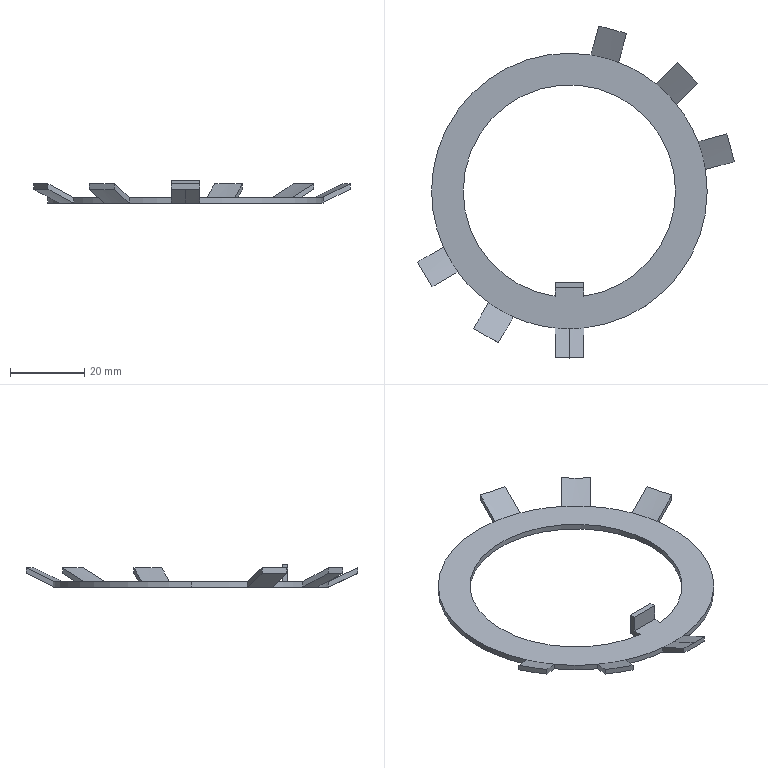Part | SolidWorks | features Boss 1, Cut 1, Revolution 1 | 1 solid | 49 faces | box 85.057 x 89.139 x 6 mm | volume 3268 mm3 | plane 25 | cone 14 | cylinder 10 | commonest cylinder face diameters 74 x7 57 x3
STEP:
#1=CARTESIAN_POINT('',(0.,-37.,0.));
#2=VERTEX_POINT('',#1);
#3=CARTESIAN_POINT('',(-3.85,-36.799,0.));
#4=VERTEX_POINT('',#3);
#5=CARTESIAN_POINT('',(0.,0.,0.));
#6=DIRECTION('',(0.,0.,-1.));
#7=DIRECTION('',(0.,1.,0.));
#8=AXIS2_PLACEMENT_3D('',#5,#6,#7);
#9=CIRCLE('',#8,37.);
#10=EDGE_CURVE('',#2,#4,#9,.T.);
#11=ORIENTED_EDGE('',*,*,#10,.F.);
#12=CARTESIAN_POINT('',(0.,-44.835,3.654));
#13=VERTEX_POINT('',#12);
#14=CARTESIAN_POINT('',(0.,-37.,0.));
#15=DIRECTION('',(0.,-0.9063,0.4226));
#16=VECTOR('',#15,1000.);
#17=LINE('',#14,#16);
#18=EDGE_CURVE('',#2,#13,#17,.T.);
#19=ORIENTED_EDGE('',*,*,#18,.T.);
#20=CARTESIAN_POINT('',(-3.85,-44.835,3.73));
#21=VERTEX_POINT('',#20);
#22=CARTESIAN_POINT('',(0.,-44.835,3.654));
#23=CARTESIAN_POINT('',(-1.282,-44.835,3.654));
#24=CARTESIAN_POINT('',(-2.567,-44.835,3.679));
#25=CARTESIAN_POINT('',(-3.85,-44.835,3.73));
#26=B_SPLINE_CURVE_WITH_KNOTS('',3,(#22,#23,#24,#25),.UNSPECIFIED.,.F.,.F.,(4,4),(0.01424,0.01808),.UNSPECIFIED.);
#27=EDGE_CURVE('',#13,#21,#26,.T.);
#28=ORIENTED_EDGE('',*,*,#27,.T.);
#29=CARTESIAN_POINT('',(-3.85,-44.835,3.73));
#30=CARTESIAN_POINT('',(-3.85,-42.157,2.486));
#31=CARTESIAN_POINT('',(-3.85,-39.478,1.242));
#32=CARTESIAN_POINT('',(-3.85,-36.799,0.));
#33=B_SPLINE_CURVE_WITH_KNOTS('',3,(#29,#30,#31,#32),.UNSPECIFIED.,.F.,.F.,(4,4),(0.01637,0.02523),.UNSPECIFIED.);
#34=EDGE_CURVE('',#21,#4,#33,.T.);
#35=ORIENTED_EDGE('',*,*,#34,.T.);
#36=EDGE_LOOP('',(#11,#19,#28,#35));
#37=FACE_OUTER_BOUND('',#36,.T.);
#38=CARTESIAN_POINT('',(0.,0.,0.));
#39=DIRECTION('',(0.,0.,1.));
#40=DIRECTION('',(0.,-1.,0.));
#41=AXIS2_PLACEMENT_3D('',#38,#39,#40);
#42=CONICAL_SURFACE('',#41,37.,1.134);
#43=ADVANCED_FACE('',(#37),#42,.T.);
#44=CARTESIAN_POINT('',(-33.794,-15.065,1.5));
#45=VERTEX_POINT('',#44);
#46=CARTESIAN_POINT('',(-37.,0.,1.5));
#47=VERTEX_POINT('',#46);
#48=CARTESIAN_POINT('',(0.,0.,1.5));
#49=DIRECTION('',(0.,0.,-1.));
#50=DIRECTION('',(0.,1.,0.));
#51=AXIS2_PLACEMENT_3D('',#48,#49,#50);
#52=CIRCLE('',#51,37.);
#53=EDGE_CURVE('',#45,#47,#52,.T.);
#54=ORIENTED_EDGE('',*,*,#53,.T.);
#55=CARTESIAN_POINT('',(-37.,0.,0.));
#56=VERTEX_POINT('',#55);
#57=CARTESIAN_POINT('',(-37.,0.,5.231));
#58=DIRECTION('',(0.,0.,-1.));
#59=VECTOR('',#58,1000.);
#60=LINE('',#57,#59);
#61=EDGE_CURVE('',#47,#56,#60,.T.);
#62=ORIENTED_EDGE('',*,*,#61,.T.);
#63=CARTESIAN_POINT('',(-33.794,-15.065,0.));
#64=VERTEX_POINT('',#63);
#65=CARTESIAN_POINT('',(0.,0.,0.));
#66=DIRECTION('',(0.,0.,1.));
#67=DIRECTION('',(1.,0.,0.));
#68=AXIS2_PLACEMENT_3D('',#65,#66,#67);
#69=CIRCLE('',#68,37.);
#70=EDGE_CURVE('',#56,#64,#69,.T.);
#71=ORIENTED_EDGE('',*,*,#70,.T.);
#72=CARTESIAN_POINT('',(-33.794,-15.065,5.231));
#73=DIRECTION('',(0.,0.,-1.));
#74=VECTOR('',#73,1000.);
#75=LINE('',#72,#74);
#76=EDGE_CURVE('',#45,#64,#75,.T.);
#77=ORIENTED_EDGE('',*,*,#76,.F.);
#78=EDGE_LOOP('',(#54,#62,#71,#77));
#79=FACE_OUTER_BOUND('',#78,.T.);
#80=CARTESIAN_POINT('',(0.,0.,5.231));
#81=DIRECTION('',(0.,0.,-1.));
#82=DIRECTION('',(-1.,0.,0.));
#83=AXIS2_PLACEMENT_3D('',#80,#81,#82);
#84=CYLINDRICAL_SURFACE('',#83,37.);
#85=ADVANCED_FACE('',(#79),#84,.T.);
#86=CARTESIAN_POINT('',(3.85,-28.239,1.5));
#87=VERTEX_POINT('',#86);
#88=CARTESIAN_POINT('',(28.5,0.,1.5));
#89=VERTEX_POINT('',#88);
#90=CARTESIAN_POINT('',(0.,0.,1.5));
#91=DIRECTION('',(0.,0.,1.));
#92=DIRECTION('',(0.,-1.,0.));
#93=AXIS2_PLACEMENT_3D('',#90,#91,#92);
#94=CIRCLE('',#93,28.5);
#95=EDGE_CURVE('',#87,#89,#94,.T.);
#96=ORIENTED_EDGE('',*,*,#95,.T.);
#97=CARTESIAN_POINT('',(28.5,0.,0.));
#98=VERTEX_POINT('',#97);
#99=CARTESIAN_POINT('',(28.5,0.,5.231));
#100=DIRECTION('',(0.,0.,-1.));
#101=VECTOR('',#100,1000.);
#102=LINE('',#99,#101);
#103=EDGE_CURVE('',#89,#98,#102,.T.);
#104=ORIENTED_EDGE('',*,*,#103,.T.);
#105=CARTESIAN_POINT('',(3.85,-28.239,0.));
#106=VERTEX_POINT('',#105);
#107=CARTESIAN_POINT('',(0.,0.,0.));
#108=DIRECTION('',(0.,0.,1.));
#109=DIRECTION('',(1.,0.,0.));
#110=AXIS2_PLACEMENT_3D('',#107,#108,#109);
#111=CIRCLE('',#110,28.5);
#112=EDGE_CURVE('',#106,#98,#111,.T.);
#113=ORIENTED_EDGE('',*,*,#112,.F.);
#114=CARTESIAN_POINT('',(3.85,-28.239,5.231));
#115=DIRECTION('',(0.,0.,-1.));
#116=VECTOR('',#115,1000.);
#117=LINE('',#114,#116);
#118=EDGE_CURVE('',#87,#106,#117,.T.);
#119=ORIENTED_EDGE('',*,*,#118,.F.);
#120=EDGE_LOOP('',(#96,#104,#113,#119));
#121=FACE_OUTER_BOUND('',#120,.T.);
#122=CARTESIAN_POINT('',(0.,0.,5.231));
#123=DIRECTION('',(0.,0.,-1.));
#124=DIRECTION('',(-1.,0.,0.));
#125=AXIS2_PLACEMENT_3D('',#122,#123,#124);
#126=CYLINDRICAL_SURFACE('',#125,28.5);
#127=ADVANCED_FACE('',(#121),#126,.F.);
#128=ORIENTED_EDGE('',*,*,#103,.F.);
#129=CARTESIAN_POINT('',(-28.5,0.,1.5));
#130=VERTEX_POINT('',#129);
#131=CARTESIAN_POINT('',(0.,0.,1.5));
#132=DIRECTION('',(0.,0.,1.));
#133=DIRECTION('',(0.,-1.,0.));
#134=AXIS2_PLACEMENT_3D('',#131,#132,#133);
#135=CIRCLE('',#134,28.5);
#136=EDGE_CURVE('',#89,#130,#135,.T.);
#137=ORIENTED_EDGE('',*,*,#136,.T.);
#138=CARTESIAN_POINT('',(-28.5,0.,0.));
#139=VERTEX_POINT('',#138);
#140=CARTESIAN_POINT('',(-28.5,0.,5.231));
#141=DIRECTION('',(0.,0.,-1.));
#142=VECTOR('',#141,1000.);
#143=LINE('',#140,#142);
#144=EDGE_CURVE('',#130,#139,#143,.T.);
#145=ORIENTED_EDGE('',*,*,#144,.T.);
#146=CARTESIAN_POINT('',(0.,0.,0.));
#147=DIRECTION('',(0.,0.,1.));
#148=DIRECTION('',(1.,0.,0.));
#149=AXIS2_PLACEMENT_3D('',#146,#147,#148);
#150=CIRCLE('',#149,28.5);
#151=EDGE_CURVE('',#98,#139,#150,.T.);
#152=ORIENTED_EDGE('',*,*,#151,.F.);
#153=EDGE_LOOP('',(#128,#137,#145,#152));
#154=FACE_OUTER_BOUND('',#153,.T.);
#155=CARTESIAN_POINT('',(0.,0.,5.231));
#156=DIRECTION('',(0.,0.,-1.));
#157=DIRECTION('',(-1.,0.,0.));
#158=AXIS2_PLACEMENT_3D('',#155,#156,#157);
#159=CYLINDRICAL_SURFACE('',#158,28.5);
#160=ADVANCED_FACE('',(#154),#159,.F.);
#161=CARTESIAN_POINT('',(3.85,-36.799,1.5));
#162=VERTEX_POINT('',#161);
#163=CARTESIAN_POINT('',(0.,-37.,1.5));
#164=VERTEX_POINT('',#163);
#165=CARTESIAN_POINT('',(0.,0.,1.5));
#166=DIRECTION('',(0.,0.,-1.));
#167=DIRECTION('',(0.,1.,0.));
#168=AXIS2_PLACEMENT_3D('',#165,#166,#167);
#169=CIRCLE('',#168,37.);
#170=EDGE_CURVE('',#162,#164,#169,.T.);
#171=ORIENTED_EDGE('',*,*,#170,.T.);
#172=CARTESIAN_POINT('',(0.,-44.835,5.154));
#173=VERTEX_POINT('',#172);
#174=CARTESIAN_POINT('',(0.,-45.,5.23));
#175=DIRECTION('',(0.,-0.9063,0.4226));
#176=VECTOR('',#175,1000.);
#177=LINE('',#174,#176);
#178=EDGE_CURVE('',#164,#173,#177,.T.);
#179=ORIENTED_EDGE('',*,*,#178,.T.);
#180=CARTESIAN_POINT('',(3.85,-44.835,5.23));
#181=VERTEX_POINT('',#180);
#182=CARTESIAN_POINT('',(0.,-44.835,5.154));
#183=CARTESIAN_POINT('',(1.285,-44.835,5.154));
#184=CARTESIAN_POINT('',(2.568,-44.835,5.179));
#185=CARTESIAN_POINT('',(3.85,-44.835,5.23));
#186=B_SPLINE_CURVE_WITH_KNOTS('',3,(#182,#183,#184,#185),.UNSPECIFIED.,.F.,.F.,(4,4),(0.01994,0.02379),.UNSPECIFIED.);
#187=EDGE_CURVE('',#173,#181,#186,.T.);
#188=ORIENTED_EDGE('',*,*,#187,.T.);
#189=CARTESIAN_POINT('',(3.85,-44.835,5.23));
#190=CARTESIAN_POINT('',(3.85,-42.157,3.986));
#191=CARTESIAN_POINT('',(3.85,-39.478,2.742));
#192=CARTESIAN_POINT('',(3.85,-36.799,1.5));
#193=B_SPLINE_CURVE_WITH_KNOTS('',3,(#189,#190,#191,#192),.UNSPECIFIED.,.F.,.F.,(4,4),(0.01637,0.02523),.UNSPECIFIED.);
#194=EDGE_CURVE('',#181,#162,#193,.T.);
#195=ORIENTED_EDGE('',*,*,#194,.T.);
#196=EDGE_LOOP('',(#171,#179,#188,#195));
#197=FACE_OUTER_BOUND('',#196,.T.);
#198=CARTESIAN_POINT('',(0.,0.,5.23));
#199=DIRECTION('',(0.,0.,1.));
#200=DIRECTION('',(0.,-1.,0.));
#201=AXIS2_PLACEMENT_3D('',#198,#199,#200);
#202=CONICAL_SURFACE('',#201,45.,1.134);
#203=ADVANCED_FACE('',(#197),#202,.F.);
#204=CARTESIAN_POINT('',(5.806,36.542,1.5));
#205=VERTEX_POINT('',#204);
#206=CARTESIAN_POINT('',(13.243,34.549,1.5));
#207=VERTEX_POINT('',#206);
#208=CARTESIAN_POINT('',(0.,0.,1.5));
#209=DIRECTION('',(0.,0.,-1.));
#210=DIRECTION('',(0.,1.,0.));
#211=AXIS2_PLACEMENT_3D('',#208,#209,#210);
#212=CIRCLE('',#211,37.);
#213=EDGE_CURVE('',#205,#207,#212,.T.);
#214=ORIENTED_EDGE('',*,*,#213,.F.);
#215=CARTESIAN_POINT('',(0.,0.,1.5));
#216=DIRECTION('',(0.,0.,-1.));
#217=DIRECTION('',(0.,1.,0.));
#218=AXIS2_PLACEMENT_3D('',#215,#216,#217);
#219=CIRCLE('',#218,37.);
#220=EDGE_CURVE('',#47,#205,#219,.T.);
#221=ORIENTED_EDGE('',*,*,#220,.F.);
#222=ORIENTED_EDGE('',*,*,#53,.F.);
#223=CARTESIAN_POINT('',(-29.944,-21.734,1.5));
#224=VERTEX_POINT('',#223);
#225=CARTESIAN_POINT('',(0.,0.,1.5));
#226=DIRECTION('',(0.,0.,-1.));
#227=DIRECTION('',(0.,1.,0.));
#228=AXIS2_PLACEMENT_3D('',#225,#226,#227);
#229=CIRCLE('',#228,37.);
#230=EDGE_CURVE('',#224,#45,#229,.T.);
#231=ORIENTED_EDGE('',*,*,#230,.F.);
#232=CARTESIAN_POINT('',(-21.734,-29.944,1.5));
#233=VERTEX_POINT('',#232);
#234=CARTESIAN_POINT('',(0.,0.,1.5));
#235=DIRECTION('',(0.,0.,-1.));
#236=DIRECTION('',(0.,1.,0.));
#237=AXIS2_PLACEMENT_3D('',#234,#235,#236);
#238=CIRCLE('',#237,37.);
#239=EDGE_CURVE('',#233,#224,#238,.T.);
#240=ORIENTED_EDGE('',*,*,#239,.F.);
#241=CARTESIAN_POINT('',(-15.065,-33.794,1.5));
#242=VERTEX_POINT('',#241);
#243=CARTESIAN_POINT('',(0.,0.,1.5));
#244=DIRECTION('',(0.,0.,-1.));
#245=DIRECTION('',(0.,1.,0.));
#246=AXIS2_PLACEMENT_3D('',#243,#244,#245);
#247=CIRCLE('',#246,37.);
#248=EDGE_CURVE('',#242,#233,#247,.T.);
#249=ORIENTED_EDGE('',*,*,#248,.F.);
#250=CARTESIAN_POINT('',(-3.85,-36.799,1.5));
#251=VERTEX_POINT('',#250);
#252=CARTESIAN_POINT('',(0.,0.,1.5));
#253=DIRECTION('',(0.,0.,-1.));
#254=DIRECTION('',(0.,1.,0.));
#255=AXIS2_PLACEMENT_3D('',#252,#253,#254);
#256=CIRCLE('',#255,37.);
#257=EDGE_CURVE('',#251,#242,#256,.T.);
#258=ORIENTED_EDGE('',*,*,#257,.F.);
#259=CARTESIAN_POINT('',(0.,0.,1.5));
#260=DIRECTION('',(0.,0.,-1.));
#261=DIRECTION('',(0.,1.,0.));
#262=AXIS2_PLACEMENT_3D('',#259,#260,#261);
#263=CIRCLE('',#262,37.);
#264=EDGE_CURVE('',#164,#251,#263,.T.);
#265=ORIENTED_EDGE('',*,*,#264,.F.);
#266=ORIENTED_EDGE('',*,*,#170,.F.);
#267=CARTESIAN_POINT('',(36.542,5.806,1.5));
#268=VERTEX_POINT('',#267);
#269=CARTESIAN_POINT('',(0.,0.,1.5));
#270=DIRECTION('',(0.,0.,-1.));
#271=DIRECTION('',(0.,1.,0.));
#272=AXIS2_PLACEMENT_3D('',#269,#270,#271);
#273=CIRCLE('',#272,37.);
#274=EDGE_CURVE('',#268,#162,#273,.T.);
#275=ORIENTED_EDGE('',*,*,#274,.F.);
#276=CARTESIAN_POINT('',(34.549,13.243,1.5));
#277=VERTEX_POINT('',#276);
#278=CARTESIAN_POINT('',(0.,0.,1.5));
#279=DIRECTION('',(0.,0.,-1.));
#280=DIRECTION('',(0.,1.,0.));
#281=AXIS2_PLACEMENT_3D('',#278,#279,#280);
#282=CIRCLE('',#281,37.);
#283=EDGE_CURVE('',#277,#268,#282,.T.);
#284=ORIENTED_EDGE('',*,*,#283,.F.);
#285=CARTESIAN_POINT('',(28.743,23.299,1.5));
#286=VERTEX_POINT('',#285);
#287=CARTESIAN_POINT('',(0.,0.,1.5));
#288=DIRECTION('',(0.,0.,-1.));
#289=DIRECTION('',(0.,1.,0.));
#290=AXIS2_PLACEMENT_3D('',#287,#288,#289);
#291=CIRCLE('',#290,37.);
#292=EDGE_CURVE('',#286,#277,#291,.T.);
#293=ORIENTED_EDGE('',*,*,#292,.F.);
#294=CARTESIAN_POINT('',(23.299,28.743,1.5));
#295=VERTEX_POINT('',#294);
#296=CARTESIAN_POINT('',(0.,0.,1.5));
#297=DIRECTION('',(0.,0.,-1.));
#298=DIRECTION('',(0.,1.,0.));
#299=AXIS2_PLACEMENT_3D('',#296,#297,#298);
#300=CIRCLE('',#299,37.);
#301=EDGE_CURVE('',#295,#286,#300,.T.);
#302=ORIENTED_EDGE('',*,*,#301,.F.);
#303=CARTESIAN_POINT('',(0.,0.,1.5));
#304=DIRECTION('',(0.,0.,-1.));
#305=DIRECTION('',(0.,1.,0.));
#306=AXIS2_PLACEMENT_3D('',#303,#304,#305);
#307=CIRCLE('',#306,37.);
#308=EDGE_CURVE('',#207,#295,#307,.T.);
#309=ORIENTED_EDGE('',*,*,#308,.F.);
#310=EDGE_LOOP('',(#214,#221,#222,#231,#240,#249,#258,#265,#266,#275,#284,#293,#302,#309));
#311=FACE_OUTER_BOUND('',#310,.T.);
#312=CARTESIAN_POINT('',(3.85,-26.,1.5));
#313=VERTEX_POINT('',#312);
#314=CARTESIAN_POINT('',(3.85,-28.239,1.5));
#315=DIRECTION('',(0.,-1.,0.));
#316=VECTOR('',#315,1000.);
#317=LINE('',#314,#316);
#318=EDGE_CURVE('',#313,#87,#317,.T.);
#319=ORIENTED_EDGE('',*,*,#318,.F.);
#320=CARTESIAN_POINT('',(-3.85,-26.,1.5));
#321=VERTEX_POINT('',#320);
#322=CARTESIAN_POINT('',(0.,-26.,1.5));
#323=DIRECTION('',(-1.,0.,0.));
#324=VECTOR('',#323,1000.);
#325=LINE('',#322,#324);
#326=EDGE_CURVE('',#313,#321,#325,.T.);
#327=ORIENTED_EDGE('',*,*,#326,.T.);
#328=CARTESIAN_POINT('',(-3.85,-28.239,1.5));
#329=VERTEX_POINT('',#328);
#330=CARTESIAN_POINT('',(-3.85,-28.239,1.5));
#331=DIRECTION('',(0.,1.,0.));
#332=VECTOR('',#331,1000.);
#333=LINE('',#330,#332);
#334=EDGE_CURVE('',#329,#321,#333,.T.);
#335=ORIENTED_EDGE('',*,*,#334,.F.);
#336=CARTESIAN_POINT('',(0.,0.,1.5));
#337=DIRECTION('',(0.,0.,1.));
#338=DIRECTION('',(0.,-1.,0.));
#339=AXIS2_PLACEMENT_3D('',#336,#337,#338);
#340=CIRCLE('',#339,28.5);
#341=EDGE_CURVE('',#130,#329,#340,.T.);
#342=ORIENTED_EDGE('',*,*,#341,.F.);
#343=ORIENTED_EDGE('',*,*,#136,.F.);
#344=ORIENTED_EDGE('',*,*,#95,.F.);
#345=EDGE_LOOP('',(#319,#327,#335,#342,#343,#344));
#346=FACE_BOUND('',#345,.T.);
#347=CARTESIAN_POINT('',(0.,37.,1.5));
#348=DIRECTION('',(0.,0.,1.));
#349=DIRECTION('',(0.,-1.,0.));
#350=AXIS2_PLACEMENT_3D('',#347,#348,#349);
#351=PLANE('',#350);
#352=ADVANCED_FACE('',(#311,#346),#351,.T.);
#353=ORIENTED_EDGE('',*,*,#178,.F.);
#354=ORIENTED_EDGE('',*,*,#264,.T.);
#355=CARTESIAN_POINT('',(-3.85,-44.835,5.23));
#356=VERTEX_POINT('',#355);
#357=CARTESIAN_POINT('',(-3.85,-36.799,1.5));
#358=CARTESIAN_POINT('',(-3.85,-39.478,2.742));
#359=CARTESIAN_POINT('',(-3.85,-42.157,3.986));
#360=CARTESIAN_POINT('',(-3.85,-44.835,5.23));
#361=B_SPLINE_CURVE_WITH_KNOTS('',3,(#357,#358,#359,#360),.UNSPECIFIED.,.F.,.F.,(4,4),(0.01012,0.01898),.UNSPECIFIED.);
#362=EDGE_CURVE('',#251,#356,#361,.T.);
#363=ORIENTED_EDGE('',*,*,#362,.T.);
#364=CARTESIAN_POINT('',(-3.85,-44.835,5.23));
#365=CARTESIAN_POINT('',(-2.567,-44.835,5.179));
#366=CARTESIAN_POINT('',(-1.282,-44.835,5.154));
#367=CARTESIAN_POINT('',(0.,-44.835,5.154));
#368=B_SPLINE_CURVE_WITH_KNOTS('',3,(#364,#365,#366,#367),.UNSPECIFIED.,.F.,.F.,(4,4),(0.0161,0.01994),.UNSPECIFIED.);
#369=EDGE_CURVE('',#356,#173,#368,.T.);
#370=ORIENTED_EDGE('',*,*,#369,.T.);
#371=EDGE_LOOP('',(#353,#354,#363,#370));
#372=FACE_OUTER_BOUND('',#371,.T.);
#373=CARTESIAN_POINT('',(0.,0.,5.23));
#374=DIRECTION('',(0.,0.,1.));
#375=DIRECTION('',(0.,-1.,0.));
#376=AXIS2_PLACEMENT_3D('',#373,#374,#375);
#377=CONICAL_SURFACE('',#376,45.,1.134);
#378=ADVANCED_FACE('',(#372),#377,.F.);
#379=CARTESIAN_POINT('',(-25.752,-36.903,5.23));
#380=VERTEX_POINT('',#379);
#381=CARTESIAN_POINT('',(-21.734,-29.944,1.5));
#382=CARTESIAN_POINT('',(-23.073,-32.264,2.742));
#383=CARTESIAN_POINT('',(-24.413,-34.584,3.986));
#384=CARTESIAN_POINT('',(-25.752,-36.903,5.23));
#385=B_SPLINE_CURVE_WITH_KNOTS('',3,(#381,#382,#383,#384),.UNSPECIFIED.,.F.,.F.,(4,4),(0.000000255,0.00886),.UNSPECIFIED.);
#386=EDGE_CURVE('',#233,#380,#385,.T.);
#387=ORIENTED_EDGE('',*,*,#386,.T.);
#388=CARTESIAN_POINT('',(-19.083,-40.753,5.23));
#389=VERTEX_POINT('',#388);
#390=CARTESIAN_POINT('',(-25.752,-36.903,5.23));
#391=CARTESIAN_POINT('',(-23.529,-38.187,5.128));
#392=CARTESIAN_POINT('',(-21.306,-39.47,5.128));
#393=CARTESIAN_POINT('',(-19.083,-40.753,5.23));
#394=B_SPLINE_CURVE_WITH_KNOTS('',3,(#390,#391,#392,#393),.UNSPECIFIED.,.F.,.F.,(4,4),(0.000000231,0.0077),.UNSPECIFIED.);
#395=EDGE_CURVE('',#380,#389,#394,.T.);
#396=ORIENTED_EDGE('',*,*,#395,.T.);
#397=CARTESIAN_POINT('',(-19.083,-40.753,5.23));
#398=CARTESIAN_POINT('',(-17.744,-38.434,3.986));
#399=CARTESIAN_POINT('',(-16.405,-36.114,2.742));
#400=CARTESIAN_POINT('',(-15.065,-33.794,1.5));
#401=B_SPLINE_CURVE_WITH_KNOTS('',3,(#397,#398,#399,#400),.UNSPECIFIED.,.F.,.F.,(4,4),(0.000000255,0.00886),.UNSPECIFIED.);
#402=EDGE_CURVE('',#389,#242,#401,.T.);
#403=ORIENTED_EDGE('',*,*,#402,.T.);
#404=ORIENTED_EDGE('',*,*,#248,.T.);
#405=EDGE_LOOP('',(#387,#396,#403,#404));
#406=FACE_OUTER_BOUND('',#405,.T.);
#407=CARTESIAN_POINT('',(0.,0.,5.23));
#408=DIRECTION('',(0.,0.,1.));
#409=DIRECTION('',(0.,-1.,0.));
#410=AXIS2_PLACEMENT_3D('',#407,#408,#409);
#411=CONICAL_SURFACE('',#410,45.,1.134);
#412=ADVANCED_FACE('',(#406),#411,.F.);
#413=CARTESIAN_POINT('',(-40.753,-19.083,5.23));
#414=VERTEX_POINT('',#413);
#415=CARTESIAN_POINT('',(-33.794,-15.065,1.5));
#416=CARTESIAN_POINT('',(-36.114,-16.405,2.742));
#417=CARTESIAN_POINT('',(-38.434,-17.744,3.986));
#418=CARTESIAN_POINT('',(-40.753,-19.083,5.23));
#419=B_SPLINE_CURVE_WITH_KNOTS('',3,(#415,#416,#417,#418),.UNSPECIFIED.,.F.,.F.,(4,4),(0.000000255,0.00886),.UNSPECIFIED.);
#420=EDGE_CURVE('',#45,#414,#419,.T.);
#421=ORIENTED_EDGE('',*,*,#420,.T.);
#422=CARTESIAN_POINT('',(-36.903,-25.752,5.23));
#423=VERTEX_POINT('',#422);
#424=CARTESIAN_POINT('',(-40.753,-19.083,5.23));
#425=CARTESIAN_POINT('',(-39.47,-21.306,5.128));
#426=CARTESIAN_POINT('',(-38.187,-23.529,5.128));
#427=CARTESIAN_POINT('',(-36.903,-25.752,5.23));
#428=B_SPLINE_CURVE_WITH_KNOTS('',3,(#424,#425,#426,#427),.UNSPECIFIED.,.F.,.F.,(4,4),(0.000000231,0.0077),.UNSPECIFIED.);
#429=EDGE_CURVE('',#414,#423,#428,.T.);
#430=ORIENTED_EDGE('',*,*,#429,.T.);
#431=CARTESIAN_POINT('',(-36.903,-25.752,5.23));
#432=CARTESIAN_POINT('',(-34.584,-24.413,3.986));
#433=CARTESIAN_POINT('',(-32.264,-23.073,2.742));
#434=CARTESIAN_POINT('',(-29.944,-21.734,1.5));
#435=B_SPLINE_CURVE_WITH_KNOTS('',3,(#431,#432,#433,#434),.UNSPECIFIED.,.F.,.F.,(4,4),(0.000000255,0.00886),.UNSPECIFIED.);
#436=EDGE_CURVE('',#423,#224,#435,.T.);
#437=ORIENTED_EDGE('',*,*,#436,.T.);
#438=ORIENTED_EDGE('',*,*,#230,.T.);
#439=EDGE_LOOP('',(#421,#430,#437,#438));
#440=FACE_OUTER_BOUND('',#439,.T.);
#441=CARTESIAN_POINT('',(0.,0.,5.23));
#442=DIRECTION('',(0.,0.,1.));
#443=DIRECTION('',(0.,-1.,0.));
#444=AXIS2_PLACEMENT_3D('',#441,#442,#443);
#445=CONICAL_SURFACE('',#444,45.,1.134);
#446=ADVANCED_FACE('',(#440),#445,.F.);
#447=CARTESIAN_POINT('',(15.323,42.311,5.23));
#448=VERTEX_POINT('',#447);
#449=CARTESIAN_POINT('',(13.243,34.549,1.5));
#450=CARTESIAN_POINT('',(13.937,37.137,2.742));
#451=CARTESIAN_POINT('',(14.63,39.724,3.986));
#452=CARTESIAN_POINT('',(15.323,42.311,5.23));
#453=B_SPLINE_CURVE_WITH_KNOTS('',3,(#449,#450,#451,#452),.UNSPECIFIED.,.F.,.F.,(4,4),(0.000000228,0.00886),.UNSPECIFIED.);
#454=EDGE_CURVE('',#207,#448,#453,.T.);
#455=ORIENTED_EDGE('',*,*,#454,.T.);
#456=CARTESIAN_POINT('',(7.885,44.304,5.23));
#457=VERTEX_POINT('',#456);
#458=CARTESIAN_POINT('',(15.323,42.311,5.23));
#459=CARTESIAN_POINT('',(12.844,42.975,5.128));
#460=CARTESIAN_POINT('',(10.365,43.639,5.128));
#461=CARTESIAN_POINT('',(7.885,44.304,5.23));
#462=B_SPLINE_CURVE_WITH_KNOTS('',3,(#458,#459,#460,#461),.UNSPECIFIED.,.F.,.F.,(4,4),(0.000000207,0.0077),.UNSPECIFIED.);
#463=EDGE_CURVE('',#448,#457,#462,.T.);
#464=ORIENTED_EDGE('',*,*,#463,.T.);
#465=CARTESIAN_POINT('',(7.885,44.304,5.23));
#466=CARTESIAN_POINT('',(7.192,41.717,3.986));
#467=CARTESIAN_POINT('',(6.499,39.129,2.742));
#468=CARTESIAN_POINT('',(5.806,36.542,1.5));
#469=B_SPLINE_CURVE_WITH_KNOTS('',3,(#465,#466,#467,#468),.UNSPECIFIED.,.F.,.F.,(4,4),(0.000000228,0.00886),.UNSPECIFIED.);
#470=EDGE_CURVE('',#457,#205,#469,.T.);
#471=ORIENTED_EDGE('',*,*,#470,.T.);
#472=ORIENTED_EDGE('',*,*,#213,.T.);
#473=EDGE_LOOP('',(#455,#464,#471,#472));
#474=FACE_OUTER_BOUND('',#473,.T.);
#475=CARTESIAN_POINT('',(0.,0.,5.23));
#476=DIRECTION('',(0.,0.,1.));
#477=DIRECTION('',(0.,-1.,0.));
#478=AXIS2_PLACEMENT_3D('',#475,#476,#477);
#479=CONICAL_SURFACE('',#478,45.,1.134);
#480=ADVANCED_FACE('',(#474),#479,.F.);
#481=CARTESIAN_POINT('',(34.425,28.981,5.23));
#482=VERTEX_POINT('',#481);
#483=CARTESIAN_POINT('',(28.743,23.299,1.5));
#484=CARTESIAN_POINT('',(30.638,25.193,2.742));
#485=CARTESIAN_POINT('',(32.532,27.087,3.986));
#486=CARTESIAN_POINT('',(34.425,28.981,5.23));
#487=B_SPLINE_CURVE_WITH_KNOTS('',3,(#483,#484,#485,#486),.UNSPECIFIED.,.F.,.F.,(4,4),(0.000000312,0.00886),.UNSPECIFIED.);
#488=EDGE_CURVE('',#286,#482,#487,.T.);
#489=ORIENTED_EDGE('',*,*,#488,.T.);
#490=CARTESIAN_POINT('',(28.981,34.425,5.23));
#491=VERTEX_POINT('',#490);
#492=CARTESIAN_POINT('',(34.425,28.981,5.23));
#493=CARTESIAN_POINT('',(32.611,30.796,5.128));
#494=CARTESIAN_POINT('',(30.796,32.611,5.128));
#495=CARTESIAN_POINT('',(28.981,34.425,5.23));
#496=B_SPLINE_CURVE_WITH_KNOTS('',3,(#492,#493,#494,#495),.UNSPECIFIED.,.F.,.F.,(4,4),(0.000000283,0.0077),.UNSPECIFIED.);
#497=EDGE_CURVE('',#482,#491,#496,.T.);
#498=ORIENTED_EDGE('',*,*,#497,.T.);
#499=CARTESIAN_POINT('',(28.981,34.425,5.23));
#500=CARTESIAN_POINT('',(27.087,32.532,3.986));
#501=CARTESIAN_POINT('',(25.193,30.638,2.742));
#502=CARTESIAN_POINT('',(23.299,28.743,1.5));
#503=B_SPLINE_CURVE_WITH_KNOTS('',3,(#499,#500,#501,#502),.UNSPECIFIED.,.F.,.F.,(4,4),(0.000000312,0.00886),.UNSPECIFIED.);
#504=EDGE_CURVE('',#491,#295,#503,.T.);
#505=ORIENTED_EDGE('',*,*,#504,.T.);
#506=ORIENTED_EDGE('',*,*,#301,.T.);
#507=EDGE_LOOP('',(#489,#498,#505,#506));
#508=FACE_OUTER_BOUND('',#507,.T.);
#509=CARTESIAN_POINT('',(0.,0.,5.23));
#510=DIRECTION('',(0.,0.,1.));
#511=DIRECTION('',(0.,-1.,0.));
#512=AXIS2_PLACEMENT_3D('',#509,#510,#511);
#513=CONICAL_SURFACE('',#512,45.,1.134);
#514=ADVANCED_FACE('',(#508),#513,.F.);
#515=CARTESIAN_POINT('',(44.304,7.885,5.23));
#516=VERTEX_POINT('',#515);
#517=CARTESIAN_POINT('',(36.542,5.806,1.5));
#518=CARTESIAN_POINT('',(39.129,6.499,2.742));
#519=CARTESIAN_POINT('',(41.717,7.192,3.986));
#520=CARTESIAN_POINT('',(44.304,7.885,5.23));
#521=B_SPLINE_CURVE_WITH_KNOTS('',3,(#517,#518,#519,#520),.UNSPECIFIED.,.F.,.F.,(4,4),(0.000000228,0.00886),.UNSPECIFIED.);
#522=EDGE_CURVE('',#268,#516,#521,.T.);
#523=ORIENTED_EDGE('',*,*,#522,.T.);
#524=CARTESIAN_POINT('',(42.311,15.323,5.23));
#525=VERTEX_POINT('',#524);
#526=CARTESIAN_POINT('',(44.304,7.885,5.23));
#527=CARTESIAN_POINT('',(43.639,10.365,5.128));
#528=CARTESIAN_POINT('',(42.975,12.844,5.128));
#529=CARTESIAN_POINT('',(42.311,15.323,5.23));
#530=B_SPLINE_CURVE_WITH_KNOTS('',3,(#526,#527,#528,#529),.UNSPECIFIED.,.F.,.F.,(4,4),(0.000000207,0.0077),.UNSPECIFIED.);
#531=EDGE_CURVE('',#516,#525,#530,.T.);
#532=ORIENTED_EDGE('',*,*,#531,.T.);
#533=CARTESIAN_POINT('',(42.311,15.323,5.23));
#534=CARTESIAN_POINT('',(39.724,14.63,3.986));
#535=CARTESIAN_POINT('',(37.137,13.937,2.742));
#536=CARTESIAN_POINT('',(34.549,13.243,1.5));
#537=B_SPLINE_CURVE_WITH_KNOTS('',3,(#533,#534,#535,#536),.UNSPECIFIED.,.F.,.F.,(4,4),(0.000000228,0.00886),.UNSPECIFIED.);
#538=EDGE_CURVE('',#525,#277,#537,.T.);
#539=ORIENTED_EDGE('',*,*,#538,.T.);
#540=ORIENTED_EDGE('',*,*,#283,.T.);
#541=EDGE_LOOP('',(#523,#532,#539,#540));
#542=FACE_OUTER_BOUND('',#541,.T.);
#543=CARTESIAN_POINT('',(0.,0.,5.23));
#544=DIRECTION('',(0.,0.,1.));
#545=DIRECTION('',(0.,-1.,0.));
#546=AXIS2_PLACEMENT_3D('',#543,#544,#545);
#547=CONICAL_SURFACE('',#546,45.,1.134);
#548=ADVANCED_FACE('',(#542),#547,.F.);
#549=CARTESIAN_POINT('',(3.85,-24.5,6.));
#550=VERTEX_POINT('',#549);
#551=CARTESIAN_POINT('',(3.85,-24.5,0.));
#552=VERTEX_POINT('',#551);
#553=CARTESIAN_POINT('',(3.85,-24.5,5.231));
#554=DIRECTION('',(0.,0.,-1.));
#555=VECTOR('',#554,1000.);
#556=LINE('',#553,#555);
#557=EDGE_CURVE('',#550,#552,#556,.T.);
#558=ORIENTED_EDGE('',*,*,#557,.F.);
#559=CARTESIAN_POINT('',(3.85,-26.,6.));
#560=VERTEX_POINT('',#559);
#561=CARTESIAN_POINT('',(3.85,-24.5,6.));
#562=DIRECTION('',(0.,1.,0.));
#563=VECTOR('',#562,1000.);
#564=LINE('',#561,#563);
#565=EDGE_CURVE('',#560,#550,#564,.T.);
#566=ORIENTED_EDGE('',*,*,#565,.F.);
#567=CARTESIAN_POINT('',(3.85,-26.,6.));
#568=DIRECTION('',(0.,0.,-1.));
#569=VECTOR('',#568,1000.);
#570=LINE('',#567,#569);
#571=EDGE_CURVE('',#560,#313,#570,.T.);
#572=ORIENTED_EDGE('',*,*,#571,.T.);
#573=ORIENTED_EDGE('',*,*,#318,.T.);
#574=ORIENTED_EDGE('',*,*,#118,.T.);
#575=CARTESIAN_POINT('',(3.85,-28.239,0.));
#576=DIRECTION('',(0.,-1.,0.));
#577=VECTOR('',#576,1000.);
#578=LINE('',#575,#577);
#579=EDGE_CURVE('',#552,#106,#578,.T.);
#580=ORIENTED_EDGE('',*,*,#579,.F.);
#581=EDGE_LOOP('',(#558,#566,#572,#573,#574,#580));
#582=FACE_OUTER_BOUND('',#581,.T.);
#583=CARTESIAN_POINT('',(3.85,-28.239,5.231));
#584=DIRECTION('',(1.,0.,0.));
#585=DIRECTION('',(0.,1.,0.));
#586=AXIS2_PLACEMENT_3D('',#583,#584,#585);
#587=PLANE('',#586);
#588=ADVANCED_FACE('',(#582),#587,.T.);
#589=CARTESIAN_POINT('',(-3.85,-24.5,6.));
#590=VERTEX_POINT('',#589);
#591=CARTESIAN_POINT('',(-3.85,-24.5,0.));
#592=VERTEX_POINT('',#591);
#593=CARTESIAN_POINT('',(-3.85,-24.5,5.231));
#594=DIRECTION('',(0.,0.,-1.));
#595=VECTOR('',#594,1000.);
#596=LINE('',#593,#595);
#597=EDGE_CURVE('',#590,#592,#596,.T.);
#598=ORIENTED_EDGE('',*,*,#597,.F.);
#599=CARTESIAN_POINT('',(-3.85,-24.5,6.));
#600=DIRECTION('',(-1.,0.,0.));
#601=VECTOR('',#600,1000.);
#602=LINE('',#599,#601);
#603=EDGE_CURVE('',#550,#590,#602,.T.);
#604=ORIENTED_EDGE('',*,*,#603,.F.);
#605=ORIENTED_EDGE('',*,*,#557,.T.);
#606=CARTESIAN_POINT('',(3.85,-24.5,0.));
#607=DIRECTION('',(1.,0.,0.));
#608=VECTOR('',#607,1000.);
#609=LINE('',#606,#608);
#610=EDGE_CURVE('',#592,#552,#609,.T.);
#611=ORIENTED_EDGE('',*,*,#610,.F.);
#612=EDGE_LOOP('',(#598,#604,#605,#611));
#613=FACE_OUTER_BOUND('',#612,.T.);
#614=CARTESIAN_POINT('',(3.85,-24.5,5.231));
#615=DIRECTION('',(0.,1.,0.));
#616=DIRECTION('',(0.,0.,1.));
#617=AXIS2_PLACEMENT_3D('',#614,#615,#616);
#618=PLANE('',#617);
#619=ADVANCED_FACE('',(#613),#618,.T.);
#620=ORIENTED_EDGE('',*,*,#597,.T.);
#621=CARTESIAN_POINT('',(-3.85,-28.239,0.));
#622=VERTEX_POINT('',#621);
#623=CARTESIAN_POINT('',(-3.85,-28.239,0.));
#624=DIRECTION('',(0.,1.,0.));
#625=VECTOR('',#624,1000.);
#626=LINE('',#623,#625);
#627=EDGE_CURVE('',#622,#592,#626,.T.);
#628=ORIENTED_EDGE('',*,*,#627,.F.);
#629=CARTESIAN_POINT('',(-3.85,-28.239,5.231));
#630=DIRECTION('',(0.,0.,-1.));
#631=VECTOR('',#630,1000.);
#632=LINE('',#629,#631);
#633=EDGE_CURVE('',#329,#622,#632,.T.);
#634=ORIENTED_EDGE('',*,*,#633,.F.);
#635=ORIENTED_EDGE('',*,*,#334,.T.);
#636=CARTESIAN_POINT('',(-3.85,-26.,6.));
#637=VERTEX_POINT('',#636);
#638=CARTESIAN_POINT('',(-3.85,-26.,6.));
#639=DIRECTION('',(0.,0.,-1.));
#640=VECTOR('',#639,1000.);
#641=LINE('',#638,#640);
#642=EDGE_CURVE('',#637,#321,#641,.T.);
#643=ORIENTED_EDGE('',*,*,#642,.F.);
#644=CARTESIAN_POINT('',(-3.85,-24.5,6.));
#645=DIRECTION('',(0.,-1.,0.));
#646=VECTOR('',#645,1000.);
#647=LINE('',#644,#646);
#648=EDGE_CURVE('',#590,#637,#647,.T.);
#649=ORIENTED_EDGE('',*,*,#648,.F.);
#650=EDGE_LOOP('',(#620,#628,#634,#635,#643,#649));
#651=FACE_OUTER_BOUND('',#650,.T.);
#652=CARTESIAN_POINT('',(-3.85,-28.239,5.231));
#653=DIRECTION('',(-1.,0.,0.));
#654=DIRECTION('',(0.,-1.,0.));
#655=AXIS2_PLACEMENT_3D('',#652,#653,#654);
#656=PLANE('',#655);
#657=ADVANCED_FACE('',(#651),#656,.T.);
#658=ORIENTED_EDGE('',*,*,#144,.F.);
#659=ORIENTED_EDGE('',*,*,#341,.T.);
#660=ORIENTED_EDGE('',*,*,#633,.T.);
#661=CARTESIAN_POINT('',(0.,0.,0.));
#662=DIRECTION('',(0.,0.,1.));
#663=DIRECTION('',(1.,0.,0.));
#664=AXIS2_PLACEMENT_3D('',#661,#662,#663);
#665=CIRCLE('',#664,28.5);
#666=EDGE_CURVE('',#139,#622,#665,.T.);
#667=ORIENTED_EDGE('',*,*,#666,.F.);
#668=EDGE_LOOP('',(#658,#659,#660,#667));
#669=FACE_OUTER_BOUND('',#668,.T.);
#670=CARTESIAN_POINT('',(0.,0.,5.231));
#671=DIRECTION('',(0.,0.,-1.));
#672=DIRECTION('',(-1.,0.,0.));
#673=AXIS2_PLACEMENT_3D('',#670,#671,#672);
#674=CYLINDRICAL_SURFACE('',#673,28.5);
#675=ADVANCED_FACE('',(#669),#674,.F.);
#676=CARTESIAN_POINT('',(3.85,-36.799,0.));
#677=VERTEX_POINT('',#676);
#678=CARTESIAN_POINT('',(3.85,-44.835,3.73));
#679=VERTEX_POINT('',#678);
#680=CARTESIAN_POINT('',(3.85,-36.799,0.));
#681=CARTESIAN_POINT('',(3.85,-39.478,1.242));
#682=CARTESIAN_POINT('',(3.85,-42.157,2.486));
#683=CARTESIAN_POINT('',(3.85,-44.835,3.73));
#684=B_SPLINE_CURVE_WITH_KNOTS('',3,(#680,#681,#682,#683),.UNSPECIFIED.,.F.,.F.,(4,4),(0.01012,0.01898),.UNSPECIFIED.);
#685=EDGE_CURVE('',#677,#679,#684,.T.);
#686=ORIENTED_EDGE('',*,*,#685,.F.);
#687=CARTESIAN_POINT('',(3.85,-36.799,5.231));
#688=DIRECTION('',(0.,0.,-1.));
#689=VECTOR('',#688,1000.);
#690=LINE('',#687,#689);
#691=EDGE_CURVE('',#162,#677,#690,.T.);
#692=ORIENTED_EDGE('',*,*,#691,.F.);
#693=ORIENTED_EDGE('',*,*,#194,.F.);
#694=CARTESIAN_POINT('',(3.85,-44.835,5.231));
#695=DIRECTION('',(0.,0.,-1.));
#696=VECTOR('',#695,1000.);
#697=LINE('',#694,#696);
#698=EDGE_CURVE('',#181,#679,#697,.T.);
#699=ORIENTED_EDGE('',*,*,#698,.T.);
#700=EDGE_LOOP('',(#686,#692,#693,#699));
#701=FACE_OUTER_BOUND('',#700,.T.);
#702=CARTESIAN_POINT('',(3.85,-36.799,5.231));
#703=DIRECTION('',(-1.,0.,0.));
#704=DIRECTION('',(0.,-1.,0.));
#705=AXIS2_PLACEMENT_3D('',#702,#703,#704);
#706=PLANE('',#705);
#707=ADVANCED_FACE('',(#701),#706,.F.);
#708=ORIENTED_EDGE('',*,*,#274,.T.);
#709=ORIENTED_EDGE('',*,*,#691,.T.);
#710=CARTESIAN_POINT('',(36.542,5.806,0.));
#711=VERTEX_POINT('',#710);
#712=CARTESIAN_POINT('',(0.,0.,0.));
#713=DIRECTION('',(0.,0.,1.));
#714=DIRECTION('',(1.,0.,0.));
#715=AXIS2_PLACEMENT_3D('',#712,#713,#714);
#716=CIRCLE('',#715,37.);
#717=EDGE_CURVE('',#677,#711,#716,.T.);
#718=ORIENTED_EDGE('',*,*,#717,.T.);
#719=CARTESIAN_POINT('',(36.542,5.806,5.231));
#720=DIRECTION('',(0.,0.,-1.));
#721=VECTOR('',#720,1000.);
#722=LINE('',#719,#721);
#723=EDGE_CURVE('',#268,#711,#722,.T.);
#724=ORIENTED_EDGE('',*,*,#723,.F.);
#725=EDGE_LOOP('',(#708,#709,#718,#724));
#726=FACE_OUTER_BOUND('',#725,.T.);
#727=CARTESIAN_POINT('',(0.,0.,5.231));
#728=DIRECTION('',(0.,0.,-1.));
#729=DIRECTION('',(-1.,0.,0.));
#730=AXIS2_PLACEMENT_3D('',#727,#728,#729);
#731=CYLINDRICAL_SURFACE('',#730,37.);
#732=ADVANCED_FACE('',(#726),#731,.T.);
#733=CARTESIAN_POINT('',(44.304,7.885,3.73));
#734=VERTEX_POINT('',#733);
#735=CARTESIAN_POINT('',(44.304,7.885,3.73));
#736=CARTESIAN_POINT('',(41.717,7.192,2.486));
#737=CARTESIAN_POINT('',(39.129,6.499,1.242));
#738=CARTESIAN_POINT('',(36.542,5.806,0.));
#739=B_SPLINE_CURVE_WITH_KNOTS('',3,(#735,#736,#737,#738),.UNSPECIFIED.,.F.,.F.,(4,4),(0.000000228,0.00886),.UNSPECIFIED.);
#740=EDGE_CURVE('',#734,#711,#739,.T.);
#741=ORIENTED_EDGE('',*,*,#740,.F.);
#742=CARTESIAN_POINT('',(44.304,7.885,5.231));
#743=DIRECTION('',(0.,0.,-1.));
#744=VECTOR('',#743,1000.);
#745=LINE('',#742,#744);
#746=EDGE_CURVE('',#516,#734,#745,.T.);
#747=ORIENTED_EDGE('',*,*,#746,.F.);
#748=ORIENTED_EDGE('',*,*,#522,.F.);
#749=ORIENTED_EDGE('',*,*,#723,.T.);
#750=EDGE_LOOP('',(#741,#747,#748,#749));
#751=FACE_OUTER_BOUND('',#750,.T.);
#752=CARTESIAN_POINT('',(36.542,5.806,5.231));
#753=DIRECTION('',(-0.2588,0.9659,0.));
#754=DIRECTION('',(-0.9659,-0.2588,0.));
#755=AXIS2_PLACEMENT_3D('',#752,#753,#754);
#756=PLANE('',#755);
#757=ADVANCED_FACE('',(#751),#756,.F.);
#758=CARTESIAN_POINT('',(42.311,15.323,3.73));
#759=VERTEX_POINT('',#758);
#760=CARTESIAN_POINT('',(42.311,15.323,3.73));
#761=CARTESIAN_POINT('',(42.975,12.844,3.628));
#762=CARTESIAN_POINT('',(43.639,10.365,3.628));
#763=CARTESIAN_POINT('',(44.304,7.885,3.73));
#764=B_SPLINE_CURVE_WITH_KNOTS('',3,(#760,#761,#762,#763),.UNSPECIFIED.,.F.,.F.,(4,4),(0.000000207,0.0077),.UNSPECIFIED.);
#765=EDGE_CURVE('',#759,#734,#764,.T.);
#766=ORIENTED_EDGE('',*,*,#765,.F.);
#767=CARTESIAN_POINT('',(42.311,15.323,5.231));
#768=DIRECTION('',(0.,0.,-1.));
#769=VECTOR('',#768,1000.);
#770=LINE('',#767,#769);
#771=EDGE_CURVE('',#525,#759,#770,.T.);
#772=ORIENTED_EDGE('',*,*,#771,.F.);
#773=ORIENTED_EDGE('',*,*,#531,.F.);
#774=ORIENTED_EDGE('',*,*,#746,.T.);
#775=EDGE_LOOP('',(#766,#772,#773,#774));
#776=FACE_OUTER_BOUND('',#775,.T.);
#777=CARTESIAN_POINT('',(42.311,15.323,5.231));
#778=DIRECTION('',(-0.9659,-0.2588,0.));
#779=DIRECTION('',(0.2588,-0.9659,0.));
#780=AXIS2_PLACEMENT_3D('',#777,#778,#779);
#781=PLANE('',#780);
#782=ADVANCED_FACE('',(#776),#781,.F.);
#783=CARTESIAN_POINT('',(34.549,13.243,0.));
#784=VERTEX_POINT('',#783);
#785=CARTESIAN_POINT('',(34.549,13.243,0.));
#786=CARTESIAN_POINT('',(37.137,13.937,1.242));
#787=CARTESIAN_POINT('',(39.724,14.63,2.486));
#788=CARTESIAN_POINT('',(42.311,15.323,3.73));
#789=B_SPLINE_CURVE_WITH_KNOTS('',3,(#785,#786,#787,#788),.UNSPECIFIED.,.F.,.F.,(4,4),(0.000000228,0.00886),.UNSPECIFIED.);
#790=EDGE_CURVE('',#784,#759,#789,.T.);
#791=ORIENTED_EDGE('',*,*,#790,.F.);
#792=CARTESIAN_POINT('',(34.549,13.243,5.231));
#793=DIRECTION('',(0.,0.,-1.));
#794=VECTOR('',#793,1000.);
#795=LINE('',#792,#794);
#796=EDGE_CURVE('',#277,#784,#795,.T.);
#797=ORIENTED_EDGE('',*,*,#796,.F.);
#798=ORIENTED_EDGE('',*,*,#538,.F.);
#799=ORIENTED_EDGE('',*,*,#771,.T.);
#800=EDGE_LOOP('',(#791,#797,#798,#799));
#801=FACE_OUTER_BOUND('',#800,.T.);
#802=CARTESIAN_POINT('',(34.549,13.243,5.231));
#803=DIRECTION('',(0.2588,-0.9659,0.));
#804=DIRECTION('',(0.9659,0.2588,0.));
#805=AXIS2_PLACEMENT_3D('',#802,#803,#804);
#806=PLANE('',#805);
#807=ADVANCED_FACE('',(#801),#806,.F.);
#808=ORIENTED_EDGE('',*,*,#292,.T.);
#809=ORIENTED_EDGE('',*,*,#796,.T.);
#810=CARTESIAN_POINT('',(28.743,23.299,0.));
#811=VERTEX_POINT('',#810);
#812=CARTESIAN_POINT('',(0.,0.,0.));
#813=DIRECTION('',(0.,0.,1.));
#814=DIRECTION('',(1.,0.,0.));
#815=AXIS2_PLACEMENT_3D('',#812,#813,#814);
#816=CIRCLE('',#815,37.);
#817=EDGE_CURVE('',#784,#811,#816,.T.);
#818=ORIENTED_EDGE('',*,*,#817,.T.);
#819=CARTESIAN_POINT('',(28.743,23.299,5.231));
#820=DIRECTION('',(0.,0.,-1.));
#821=VECTOR('',#820,1000.);
#822=LINE('',#819,#821);
#823=EDGE_CURVE('',#286,#811,#822,.T.);
#824=ORIENTED_EDGE('',*,*,#823,.F.);
#825=EDGE_LOOP('',(#808,#809,#818,#824));
#826=FACE_OUTER_BOUND('',#825,.T.);
#827=CARTESIAN_POINT('',(0.,0.,5.231));
#828=DIRECTION('',(0.,0.,-1.));
#829=DIRECTION('',(-1.,0.,0.));
#830=AXIS2_PLACEMENT_3D('',#827,#828,#829);
#831=CYLINDRICAL_SURFACE('',#830,37.);
#832=ADVANCED_FACE('',(#826),#831,.T.);
#833=CARTESIAN_POINT('',(34.425,28.981,3.73));
#834=VERTEX_POINT('',#833);
#835=CARTESIAN_POINT('',(34.425,28.981,3.73));
#836=CARTESIAN_POINT('',(32.532,27.087,2.486));
#837=CARTESIAN_POINT('',(30.638,25.193,1.242));
#838=CARTESIAN_POINT('',(28.743,23.299,0.));
#839=B_SPLINE_CURVE_WITH_KNOTS('',3,(#835,#836,#837,#838),.UNSPECIFIED.,.F.,.F.,(4,4),(0.000000312,0.00886),.UNSPECIFIED.);
#840=EDGE_CURVE('',#834,#811,#839,.T.);
#841=ORIENTED_EDGE('',*,*,#840,.F.);
#842=CARTESIAN_POINT('',(34.425,28.981,5.231));
#843=DIRECTION('',(0.,0.,-1.));
#844=VECTOR('',#843,1000.);
#845=LINE('',#842,#844);
#846=EDGE_CURVE('',#482,#834,#845,.T.);
#847=ORIENTED_EDGE('',*,*,#846,.F.);
#848=ORIENTED_EDGE('',*,*,#488,.F.);
#849=ORIENTED_EDGE('',*,*,#823,.T.);
#850=EDGE_LOOP('',(#841,#847,#848,#849));
#851=FACE_OUTER_BOUND('',#850,.T.);
#852=CARTESIAN_POINT('',(28.743,23.299,5.231));
#853=DIRECTION('',(-0.7071,0.7071,0.));
#854=DIRECTION('',(-0.7071,-0.7071,0.));
#855=AXIS2_PLACEMENT_3D('',#852,#853,#854);
#856=PLANE('',#855);
#857=ADVANCED_FACE('',(#851),#856,.F.);
#858=CARTESIAN_POINT('',(28.981,34.425,3.73));
#859=VERTEX_POINT('',#858);
#860=CARTESIAN_POINT('',(28.981,34.425,3.73));
#861=CARTESIAN_POINT('',(30.796,32.611,3.628));
#862=CARTESIAN_POINT('',(32.611,30.796,3.628));
#863=CARTESIAN_POINT('',(34.425,28.981,3.73));
#864=B_SPLINE_CURVE_WITH_KNOTS('',3,(#860,#861,#862,#863),.UNSPECIFIED.,.F.,.F.,(4,4),(0.000000283,0.0077),.UNSPECIFIED.);
#865=EDGE_CURVE('',#859,#834,#864,.T.);
#866=ORIENTED_EDGE('',*,*,#865,.F.);
#867=CARTESIAN_POINT('',(28.981,34.425,5.231));
#868=DIRECTION('',(0.,0.,-1.));
#869=VECTOR('',#868,1000.);
#870=LINE('',#867,#869);
#871=EDGE_CURVE('',#491,#859,#870,.T.);
#872=ORIENTED_EDGE('',*,*,#871,.F.);
#873=ORIENTED_EDGE('',*,*,#497,.F.);
#874=ORIENTED_EDGE('',*,*,#846,.T.);
#875=EDGE_LOOP('',(#866,#872,#873,#874));
#876=FACE_OUTER_BOUND('',#875,.T.);
#877=CARTESIAN_POINT('',(28.981,34.425,5.231));
#878=DIRECTION('',(-0.7071,-0.7071,0.));
#879=DIRECTION('',(0.7071,-0.7071,0.));
#880=AXIS2_PLACEMENT_3D('',#877,#878,#879);
#881=PLANE('',#880);
#882=ADVANCED_FACE('',(#876),#881,.F.);
#883=CARTESIAN_POINT('',(23.299,28.743,0.));
#884=VERTEX_POINT('',#883);
#885=CARTESIAN_POINT('',(23.299,28.743,0.));
#886=CARTESIAN_POINT('',(25.193,30.638,1.242));
#887=CARTESIAN_POINT('',(27.087,32.532,2.486));
#888=CARTESIAN_POINT('',(28.981,34.425,3.73));
#889=B_SPLINE_CURVE_WITH_KNOTS('',3,(#885,#886,#887,#888),.UNSPECIFIED.,.F.,.F.,(4,4),(0.000000312,0.00886),.UNSPECIFIED.);
#890=EDGE_CURVE('',#884,#859,#889,.T.);
#891=ORIENTED_EDGE('',*,*,#890,.F.);
#892=CARTESIAN_POINT('',(23.299,28.743,5.231));
#893=DIRECTION('',(0.,0.,-1.));
#894=VECTOR('',#893,1000.);
#895=LINE('',#892,#894);
#896=EDGE_CURVE('',#295,#884,#895,.T.);
#897=ORIENTED_EDGE('',*,*,#896,.F.);
#898=ORIENTED_EDGE('',*,*,#504,.F.);
#899=ORIENTED_EDGE('',*,*,#871,.T.);
#900=EDGE_LOOP('',(#891,#897,#898,#899));
#901=FACE_OUTER_BOUND('',#900,.T.);
#902=CARTESIAN_POINT('',(23.299,28.743,5.231));
#903=DIRECTION('',(0.7071,-0.7071,0.));
#904=DIRECTION('',(0.7071,0.7071,0.));
#905=AXIS2_PLACEMENT_3D('',#902,#903,#904);
#906=PLANE('',#905);
#907=ADVANCED_FACE('',(#901),#906,.F.);
#908=ORIENTED_EDGE('',*,*,#308,.T.);
#909=ORIENTED_EDGE('',*,*,#896,.T.);
#910=CARTESIAN_POINT('',(13.243,34.549,0.));
#911=VERTEX_POINT('',#910);
#912=CARTESIAN_POINT('',(0.,0.,0.));
#913=DIRECTION('',(0.,0.,1.));
#914=DIRECTION('',(1.,0.,0.));
#915=AXIS2_PLACEMENT_3D('',#912,#913,#914);
#916=CIRCLE('',#915,37.);
#917=EDGE_CURVE('',#884,#911,#916,.T.);
#918=ORIENTED_EDGE('',*,*,#917,.T.);
#919=CARTESIAN_POINT('',(13.243,34.549,5.231));
#920=DIRECTION('',(0.,0.,-1.));
#921=VECTOR('',#920,1000.);
#922=LINE('',#919,#921);
#923=EDGE_CURVE('',#207,#911,#922,.T.);
#924=ORIENTED_EDGE('',*,*,#923,.F.);
#925=EDGE_LOOP('',(#908,#909,#918,#924));
#926=FACE_OUTER_BOUND('',#925,.T.);
#927=CARTESIAN_POINT('',(0.,0.,5.231));
#928=DIRECTION('',(0.,0.,-1.));
#929=DIRECTION('',(-1.,0.,0.));
#930=AXIS2_PLACEMENT_3D('',#927,#928,#929);
#931=CYLINDRICAL_SURFACE('',#930,37.);
#932=ADVANCED_FACE('',(#926),#931,.T.);
#933=CARTESIAN_POINT('',(15.323,42.311,3.73));
#934=VERTEX_POINT('',#933);
#935=CARTESIAN_POINT('',(15.323,42.311,3.73));
#936=CARTESIAN_POINT('',(14.63,39.724,2.486));
#937=CARTESIAN_POINT('',(13.937,37.137,1.242));
#938=CARTESIAN_POINT('',(13.243,34.549,0.));
#939=B_SPLINE_CURVE_WITH_KNOTS('',3,(#935,#936,#937,#938),.UNSPECIFIED.,.F.,.F.,(4,4),(0.000000228,0.00886),.UNSPECIFIED.);
#940=EDGE_CURVE('',#934,#911,#939,.T.);
#941=ORIENTED_EDGE('',*,*,#940,.F.);
#942=CARTESIAN_POINT('',(15.323,42.311,5.231));
#943=DIRECTION('',(0.,0.,-1.));
#944=VECTOR('',#943,1000.);
#945=LINE('',#942,#944);
#946=EDGE_CURVE('',#448,#934,#945,.T.);
#947=ORIENTED_EDGE('',*,*,#946,.F.);
#948=ORIENTED_EDGE('',*,*,#454,.F.);
#949=ORIENTED_EDGE('',*,*,#923,.T.);
#950=EDGE_LOOP('',(#941,#947,#948,#949));
#951=FACE_OUTER_BOUND('',#950,.T.);
#952=CARTESIAN_POINT('',(15.323,42.311,5.231));
#953=DIRECTION('',(-0.9659,0.2588,0.));
#954=DIRECTION('',(-0.2588,-0.9659,0.));
#955=AXIS2_PLACEMENT_3D('',#952,#953,#954);
#956=PLANE('',#955);
#957=ADVANCED_FACE('',(#951),#956,.F.);
#958=CARTESIAN_POINT('',(7.885,44.304,3.73));
#959=VERTEX_POINT('',#958);
#960=CARTESIAN_POINT('',(7.885,44.304,3.73));
#961=CARTESIAN_POINT('',(10.365,43.639,3.628));
#962=CARTESIAN_POINT('',(12.844,42.975,3.628));
#963=CARTESIAN_POINT('',(15.323,42.311,3.73));
#964=B_SPLINE_CURVE_WITH_KNOTS('',3,(#960,#961,#962,#963),.UNSPECIFIED.,.F.,.F.,(4,4),(0.000000207,0.0077),.UNSPECIFIED.);
#965=EDGE_CURVE('',#959,#934,#964,.T.);
#966=ORIENTED_EDGE('',*,*,#965,.F.);
#967=CARTESIAN_POINT('',(7.885,44.304,5.231));
#968=DIRECTION('',(0.,0.,-1.));
#969=VECTOR('',#968,1000.);
#970=LINE('',#967,#969);
#971=EDGE_CURVE('',#457,#959,#970,.T.);
#972=ORIENTED_EDGE('',*,*,#971,.F.);
#973=ORIENTED_EDGE('',*,*,#463,.F.);
#974=ORIENTED_EDGE('',*,*,#946,.T.);
#975=EDGE_LOOP('',(#966,#972,#973,#974));
#976=FACE_OUTER_BOUND('',#975,.T.);
#977=CARTESIAN_POINT('',(7.885,44.304,5.231));
#978=DIRECTION('',(-0.2588,-0.9659,0.));
#979=DIRECTION('',(0.9659,-0.2588,0.));
#980=AXIS2_PLACEMENT_3D('',#977,#978,#979);
#981=PLANE('',#980);
#982=ADVANCED_FACE('',(#976),#981,.F.);
#983=CARTESIAN_POINT('',(5.806,36.542,0.));
#984=VERTEX_POINT('',#983);
#985=CARTESIAN_POINT('',(5.806,36.542,0.));
#986=CARTESIAN_POINT('',(6.499,39.129,1.242));
#987=CARTESIAN_POINT('',(7.192,41.717,2.486));
#988=CARTESIAN_POINT('',(7.885,44.304,3.73));
#989=B_SPLINE_CURVE_WITH_KNOTS('',3,(#985,#986,#987,#988),.UNSPECIFIED.,.F.,.F.,(4,4),(0.000000228,0.00886),.UNSPECIFIED.);
#990=EDGE_CURVE('',#984,#959,#989,.T.);
#991=ORIENTED_EDGE('',*,*,#990,.F.);
#992=CARTESIAN_POINT('',(5.806,36.542,5.231));
#993=DIRECTION('',(0.,0.,-1.));
#994=VECTOR('',#993,1000.);
#995=LINE('',#992,#994);
#996=EDGE_CURVE('',#205,#984,#995,.T.);
#997=ORIENTED_EDGE('',*,*,#996,.F.);
#998=ORIENTED_EDGE('',*,*,#470,.F.);
#999=ORIENTED_EDGE('',*,*,#971,.T.);
#1000=EDGE_LOOP('',(#991,#997,#998,#999));
#1001=FACE_OUTER_BOUND('',#1000,.T.);
#1002=CARTESIAN_POINT('',(7.885,44.304,5.231));
#1003=DIRECTION('',(0.9659,-0.2588,0.));
#1004=DIRECTION('',(0.2588,0.9659,0.));
#1005=AXIS2_PLACEMENT_3D('',#1002,#1003,#1004);
#1006=PLANE('',#1005);
#1007=ADVANCED_FACE('',(#1001),#1006,.F.);
#1008=ORIENTED_EDGE('',*,*,#61,.F.);
#1009=ORIENTED_EDGE('',*,*,#220,.T.);
#1010=ORIENTED_EDGE('',*,*,#996,.T.);
#1011=CARTESIAN_POINT('',(0.,0.,0.));
#1012=DIRECTION('',(0.,0.,1.));
#1013=DIRECTION('',(1.,0.,0.));
#1014=AXIS2_PLACEMENT_3D('',#1011,#1012,#1013);
#1015=CIRCLE('',#1014,37.);
#1016=EDGE_CURVE('',#984,#56,#1015,.T.);
#1017=ORIENTED_EDGE('',*,*,#1016,.T.);
#1018=EDGE_LOOP('',(#1008,#1009,#1010,#1017));
#1019=FACE_OUTER_BOUND('',#1018,.T.);
#1020=CARTESIAN_POINT('',(0.,0.,5.231));
#1021=DIRECTION('',(0.,0.,-1.));
#1022=DIRECTION('',(-1.,0.,0.));
#1023=AXIS2_PLACEMENT_3D('',#1020,#1021,#1022);
#1024=CYLINDRICAL_SURFACE('',#1023,37.);
#1025=ADVANCED_FACE('',(#1019),#1024,.T.);
#1026=CARTESIAN_POINT('',(-40.753,-19.083,3.73));
#1027=VERTEX_POINT('',#1026);
#1028=CARTESIAN_POINT('',(-40.753,-19.083,3.73));
#1029=CARTESIAN_POINT('',(-38.434,-17.744,2.486));
#1030=CARTESIAN_POINT('',(-36.114,-16.405,1.242));
#1031=CARTESIAN_POINT('',(-33.794,-15.065,0.));
#1032=B_SPLINE_CURVE_WITH_KNOTS('',3,(#1028,#1029,#1030,#1031),.UNSPECIFIED.,.F.,.F.,(4,4),(0.000000255,0.00886),.UNSPECIFIED.);
#1033=EDGE_CURVE('',#1027,#64,#1032,.T.);
#1034=ORIENTED_EDGE('',*,*,#1033,.F.);
#1035=CARTESIAN_POINT('',(-40.753,-19.083,5.231));
#1036=DIRECTION('',(0.,0.,-1.));
#1037=VECTOR('',#1036,1000.);
#1038=LINE('',#1035,#1037);
#1039=EDGE_CURVE('',#414,#1027,#1038,.T.);
#1040=ORIENTED_EDGE('',*,*,#1039,.F.);
#1041=ORIENTED_EDGE('',*,*,#420,.F.);
#1042=ORIENTED_EDGE('',*,*,#76,.T.);
#1043=EDGE_LOOP('',(#1034,#1040,#1041,#1042));
#1044=FACE_OUTER_BOUND('',#1043,.T.);
#1045=CARTESIAN_POINT('',(-33.794,-15.065,5.231));
#1046=DIRECTION('',(0.5,-0.866,0.));
#1047=DIRECTION('',(0.866,0.5,0.));
#1048=AXIS2_PLACEMENT_3D('',#1045,#1046,#1047);
#1049=PLANE('',#1048);
#1050=ADVANCED_FACE('',(#1044),#1049,.F.);
#1051=CARTESIAN_POINT('',(-36.903,-25.752,3.73));
#1052=VERTEX_POINT('',#1051);
#1053=CARTESIAN_POINT('',(-36.903,-25.752,3.73));
#1054=CARTESIAN_POINT('',(-38.187,-23.529,3.628));
#1055=CARTESIAN_POINT('',(-39.47,-21.306,3.628));
#1056=CARTESIAN_POINT('',(-40.753,-19.083,3.73));
#1057=B_SPLINE_CURVE_WITH_KNOTS('',3,(#1053,#1054,#1055,#1056),.UNSPECIFIED.,.F.,.F.,(4,4),(0.000000231,0.0077),.UNSPECIFIED.);
#1058=EDGE_CURVE('',#1052,#1027,#1057,.T.);
#1059=ORIENTED_EDGE('',*,*,#1058,.F.);
#1060=CARTESIAN_POINT('',(-36.903,-25.752,5.231));
#1061=DIRECTION('',(0.,0.,-1.));
#1062=VECTOR('',#1061,1000.);
#1063=LINE('',#1060,#1062);
#1064=EDGE_CURVE('',#423,#1052,#1063,.T.);
#1065=ORIENTED_EDGE('',*,*,#1064,.F.);
#1066=ORIENTED_EDGE('',*,*,#429,.F.);
#1067=ORIENTED_EDGE('',*,*,#1039,.T.);
#1068=EDGE_LOOP('',(#1059,#1065,#1066,#1067));
#1069=FACE_OUTER_BOUND('',#1068,.T.);
#1070=CARTESIAN_POINT('',(-36.903,-25.752,5.231));
#1071=DIRECTION('',(0.866,0.5,0.));
#1072=DIRECTION('',(-0.5,0.866,0.));
#1073=AXIS2_PLACEMENT_3D('',#1070,#1071,#1072);
#1074=PLANE('',#1073);
#1075=ADVANCED_FACE('',(#1069),#1074,.F.);
#1076=CARTESIAN_POINT('',(-29.944,-21.734,0.));
#1077=VERTEX_POINT('',#1076);
#1078=CARTESIAN_POINT('',(-29.944,-21.734,0.));
#1079=CARTESIAN_POINT('',(-32.264,-23.073,1.242));
#1080=CARTESIAN_POINT('',(-34.584,-24.413,2.486));
#1081=CARTESIAN_POINT('',(-36.903,-25.752,3.73));
#1082=B_SPLINE_CURVE_WITH_KNOTS('',3,(#1078,#1079,#1080,#1081),.UNSPECIFIED.,.F.,.F.,(4,4),(0.000000255,0.00886),.UNSPECIFIED.);
#1083=EDGE_CURVE('',#1077,#1052,#1082,.T.);
#1084=ORIENTED_EDGE('',*,*,#1083,.F.);
#1085=CARTESIAN_POINT('',(-29.944,-21.734,5.231));
#1086=DIRECTION('',(0.,0.,-1.));
#1087=VECTOR('',#1086,1000.);
#1088=LINE('',#1085,#1087);
#1089=EDGE_CURVE('',#224,#1077,#1088,.T.);
#1090=ORIENTED_EDGE('',*,*,#1089,.F.);
#1091=ORIENTED_EDGE('',*,*,#436,.F.);
#1092=ORIENTED_EDGE('',*,*,#1064,.T.);
#1093=EDGE_LOOP('',(#1084,#1090,#1091,#1092));
#1094=FACE_OUTER_BOUND('',#1093,.T.);
#1095=CARTESIAN_POINT('',(-29.944,-21.734,5.231));
#1096=DIRECTION('',(-0.5,0.866,0.));
#1097=DIRECTION('',(-0.866,-0.5,0.));
#1098=AXIS2_PLACEMENT_3D('',#1095,#1096,#1097);
#1099=PLANE('',#1098);
#1100=ADVANCED_FACE('',(#1094),#1099,.F.);
#1101=ORIENTED_EDGE('',*,*,#239,.T.);
#1102=ORIENTED_EDGE('',*,*,#1089,.T.);
#1103=CARTESIAN_POINT('',(-21.734,-29.944,0.));
#1104=VERTEX_POINT('',#1103);
#1105=CARTESIAN_POINT('',(0.,0.,0.));
#1106=DIRECTION('',(0.,0.,1.));
#1107=DIRECTION('',(1.,0.,0.));
#1108=AXIS2_PLACEMENT_3D('',#1105,#1106,#1107);
#1109=CIRCLE('',#1108,37.);
#1110=EDGE_CURVE('',#1077,#1104,#1109,.T.);
#1111=ORIENTED_EDGE('',*,*,#1110,.T.);
#1112=CARTESIAN_POINT('',(-21.734,-29.944,5.231));
#1113=DIRECTION('',(0.,0.,-1.));
#1114=VECTOR('',#1113,1000.);
#1115=LINE('',#1112,#1114);
#1116=EDGE_CURVE('',#233,#1104,#1115,.T.);
#1117=ORIENTED_EDGE('',*,*,#1116,.F.);
#1118=EDGE_LOOP('',(#1101,#1102,#1111,#1117));
#1119=FACE_OUTER_BOUND('',#1118,.T.);
#1120=CARTESIAN_POINT('',(0.,0.,5.231));
#1121=DIRECTION('',(0.,0.,-1.));
#1122=DIRECTION('',(-1.,0.,0.));
#1123=AXIS2_PLACEMENT_3D('',#1120,#1121,#1122);
#1124=CYLINDRICAL_SURFACE('',#1123,37.);
#1125=ADVANCED_FACE('',(#1119),#1124,.T.);
#1126=CARTESIAN_POINT('',(-25.752,-36.903,3.73));
#1127=VERTEX_POINT('',#1126);
#1128=CARTESIAN_POINT('',(-25.752,-36.903,3.73));
#1129=CARTESIAN_POINT('',(-24.413,-34.584,2.486));
#1130=CARTESIAN_POINT('',(-23.073,-32.264,1.242));
#1131=CARTESIAN_POINT('',(-21.734,-29.944,0.));
#1132=B_SPLINE_CURVE_WITH_KNOTS('',3,(#1128,#1129,#1130,#1131),.UNSPECIFIED.,.F.,.F.,(4,4),(0.000000255,0.00886),.UNSPECIFIED.);
#1133=EDGE_CURVE('',#1127,#1104,#1132,.T.);
#1134=ORIENTED_EDGE('',*,*,#1133,.F.);
#1135=CARTESIAN_POINT('',(-25.752,-36.903,5.231));
#1136=DIRECTION('',(0.,0.,-1.));
#1137=VECTOR('',#1136,1000.);
#1138=LINE('',#1135,#1137);
#1139=EDGE_CURVE('',#380,#1127,#1138,.T.);
#1140=ORIENTED_EDGE('',*,*,#1139,.F.);
#1141=ORIENTED_EDGE('',*,*,#386,.F.);
#1142=ORIENTED_EDGE('',*,*,#1116,.T.);
#1143=EDGE_LOOP('',(#1134,#1140,#1141,#1142));
#1144=FACE_OUTER_BOUND('',#1143,.T.);
#1145=CARTESIAN_POINT('',(-25.752,-36.903,5.231));
#1146=DIRECTION('',(0.866,-0.5,0.));
#1147=DIRECTION('',(0.5,0.866,0.));
#1148=AXIS2_PLACEMENT_3D('',#1145,#1146,#1147);
#1149=PLANE('',#1148);
#1150=ADVANCED_FACE('',(#1144),#1149,.F.);
#1151=CARTESIAN_POINT('',(-19.083,-40.753,3.73));
#1152=VERTEX_POINT('',#1151);
#1153=CARTESIAN_POINT('',(-19.083,-40.753,3.73));
#1154=CARTESIAN_POINT('',(-21.306,-39.47,3.628));
#1155=CARTESIAN_POINT('',(-23.529,-38.187,3.628));
#1156=CARTESIAN_POINT('',(-25.752,-36.903,3.73));
#1157=B_SPLINE_CURVE_WITH_KNOTS('',3,(#1153,#1154,#1155,#1156),.UNSPECIFIED.,.F.,.F.,(4,4),(0.000000231,0.0077),.UNSPECIFIED.);
#1158=EDGE_CURVE('',#1152,#1127,#1157,.T.);
#1159=ORIENTED_EDGE('',*,*,#1158,.F.);
#1160=CARTESIAN_POINT('',(-19.083,-40.753,5.231));
#1161=DIRECTION('',(0.,0.,-1.));
#1162=VECTOR('',#1161,1000.);
#1163=LINE('',#1160,#1162);
#1164=EDGE_CURVE('',#389,#1152,#1163,.T.);
#1165=ORIENTED_EDGE('',*,*,#1164,.F.);
#1166=ORIENTED_EDGE('',*,*,#395,.F.);
#1167=ORIENTED_EDGE('',*,*,#1139,.T.);
#1168=EDGE_LOOP('',(#1159,#1165,#1166,#1167));
#1169=FACE_OUTER_BOUND('',#1168,.T.);
#1170=CARTESIAN_POINT('',(-25.752,-36.903,5.231));
#1171=DIRECTION('',(0.5,0.866,0.));
#1172=DIRECTION('',(-0.866,0.5,0.));
#1173=AXIS2_PLACEMENT_3D('',#1170,#1171,#1172);
#1174=PLANE('',#1173);
#1175=ADVANCED_FACE('',(#1169),#1174,.F.);
#1176=CARTESIAN_POINT('',(-15.065,-33.794,0.));
#1177=VERTEX_POINT('',#1176);
#1178=CARTESIAN_POINT('',(-15.065,-33.794,0.));
#1179=CARTESIAN_POINT('',(-16.405,-36.114,1.242));
#1180=CARTESIAN_POINT('',(-17.744,-38.434,2.486));
#1181=CARTESIAN_POINT('',(-19.083,-40.753,3.73));
#1182=B_SPLINE_CURVE_WITH_KNOTS('',3,(#1178,#1179,#1180,#1181),.UNSPECIFIED.,.F.,.F.,(4,4),(0.000000255,0.00886),.UNSPECIFIED.);
#1183=EDGE_CURVE('',#1177,#1152,#1182,.T.);
#1184=ORIENTED_EDGE('',*,*,#1183,.F.);
#1185=CARTESIAN_POINT('',(-15.065,-33.794,5.231));
#1186=DIRECTION('',(0.,0.,-1.));
#1187=VECTOR('',#1186,1000.);
#1188=LINE('',#1185,#1187);
#1189=EDGE_CURVE('',#242,#1177,#1188,.T.);
#1190=ORIENTED_EDGE('',*,*,#1189,.F.);
#1191=ORIENTED_EDGE('',*,*,#402,.F.);
#1192=ORIENTED_EDGE('',*,*,#1164,.T.);
#1193=EDGE_LOOP('',(#1184,#1190,#1191,#1192));
#1194=FACE_OUTER_BOUND('',#1193,.T.);
#1195=CARTESIAN_POINT('',(-19.083,-40.753,5.231));
#1196=DIRECTION('',(-0.866,0.5,0.));
#1197=DIRECTION('',(-0.5,-0.866,0.));
#1198=AXIS2_PLACEMENT_3D('',#1195,#1196,#1197);
#1199=PLANE('',#1198);
#1200=ADVANCED_FACE('',(#1194),#1199,.F.);
#1201=ORIENTED_EDGE('',*,*,#257,.T.);
#1202=ORIENTED_EDGE('',*,*,#1189,.T.);
#1203=CARTESIAN_POINT('',(0.,0.,0.));
#1204=DIRECTION('',(0.,0.,1.));
#1205=DIRECTION('',(1.,0.,0.));
#1206=AXIS2_PLACEMENT_3D('',#1203,#1204,#1205);
#1207=CIRCLE('',#1206,37.);
#1208=EDGE_CURVE('',#1177,#4,#1207,.T.);
#1209=ORIENTED_EDGE('',*,*,#1208,.T.);
#1210=CARTESIAN_POINT('',(-3.85,-36.799,5.231));
#1211=DIRECTION('',(0.,0.,-1.));
#1212=VECTOR('',#1211,1000.);
#1213=LINE('',#1210,#1212);
#1214=EDGE_CURVE('',#251,#4,#1213,.T.);
#1215=ORIENTED_EDGE('',*,*,#1214,.F.);
#1216=EDGE_LOOP('',(#1201,#1202,#1209,#1215));
#1217=FACE_OUTER_BOUND('',#1216,.T.);
#1218=CARTESIAN_POINT('',(0.,0.,5.231));
#1219=DIRECTION('',(0.,0.,-1.));
#1220=DIRECTION('',(-1.,0.,0.));
#1221=AXIS2_PLACEMENT_3D('',#1218,#1219,#1220);
#1222=CYLINDRICAL_SURFACE('',#1221,37.);
#1223=ADVANCED_FACE('',(#1217),#1222,.T.);
#1224=ORIENTED_EDGE('',*,*,#34,.F.);
#1225=CARTESIAN_POINT('',(-3.85,-44.835,5.231));
#1226=DIRECTION('',(0.,0.,-1.));
#1227=VECTOR('',#1226,1000.);
#1228=LINE('',#1225,#1227);
#1229=EDGE_CURVE('',#356,#21,#1228,.T.);
#1230=ORIENTED_EDGE('',*,*,#1229,.F.);
#1231=ORIENTED_EDGE('',*,*,#362,.F.);
#1232=ORIENTED_EDGE('',*,*,#1214,.T.);
#1233=EDGE_LOOP('',(#1224,#1230,#1231,#1232));
#1234=FACE_OUTER_BOUND('',#1233,.T.);
#1235=CARTESIAN_POINT('',(-3.85,-36.799,5.231));
#1236=DIRECTION('',(1.,0.,0.));
#1237=DIRECTION('',(0.,1.,0.));
#1238=AXIS2_PLACEMENT_3D('',#1235,#1236,#1237);
#1239=PLANE('',#1238);
#1240=ADVANCED_FACE('',(#1234),#1239,.F.);
#1241=CARTESIAN_POINT('',(3.85,-44.835,3.73));
#1242=CARTESIAN_POINT('',(2.568,-44.835,3.679));
#1243=CARTESIAN_POINT('',(1.285,-44.835,3.654));
#1244=CARTESIAN_POINT('',(0.,-44.835,3.654));
#1245=B_SPLINE_CURVE_WITH_KNOTS('',3,(#1241,#1242,#1243,#1244),.UNSPECIFIED.,.F.,.F.,(4,4),(0.01039,0.01424),.UNSPECIFIED.);
#1246=EDGE_CURVE('',#679,#13,#1245,.T.);
#1247=ORIENTED_EDGE('',*,*,#1246,.F.);
#1248=ORIENTED_EDGE('',*,*,#698,.F.);
#1249=ORIENTED_EDGE('',*,*,#187,.F.);
#1250=ORIENTED_EDGE('',*,*,#369,.F.);
#1251=ORIENTED_EDGE('',*,*,#1229,.T.);
#1252=ORIENTED_EDGE('',*,*,#27,.F.);
#1253=EDGE_LOOP('',(#1247,#1248,#1249,#1250,#1251,#1252));
#1254=FACE_OUTER_BOUND('',#1253,.T.);
#1255=CARTESIAN_POINT('',(-3.85,-44.835,5.231));
#1256=DIRECTION('',(0.,1.,0.));
#1257=DIRECTION('',(0.,0.,1.));
#1258=AXIS2_PLACEMENT_3D('',#1255,#1256,#1257);
#1259=PLANE('',#1258);
#1260=ADVANCED_FACE('',(#1254),#1259,.F.);
#1261=ORIENTED_EDGE('',*,*,#740,.T.);
#1262=CARTESIAN_POINT('',(0.,0.,0.));
#1263=DIRECTION('',(0.,0.,-1.));
#1264=DIRECTION('',(0.,1.,0.));
#1265=AXIS2_PLACEMENT_3D('',#1262,#1263,#1264);
#1266=CIRCLE('',#1265,37.);
#1267=EDGE_CURVE('',#784,#711,#1266,.T.);
#1268=ORIENTED_EDGE('',*,*,#1267,.F.);
#1269=ORIENTED_EDGE('',*,*,#790,.T.);
#1270=ORIENTED_EDGE('',*,*,#765,.T.);
#1271=EDGE_LOOP('',(#1261,#1268,#1269,#1270));
#1272=FACE_OUTER_BOUND('',#1271,.T.);
#1273=CARTESIAN_POINT('',(0.,0.,0.));
#1274=DIRECTION('',(0.,0.,1.));
#1275=DIRECTION('',(0.,-1.,0.));
#1276=AXIS2_PLACEMENT_3D('',#1273,#1274,#1275);
#1277=CONICAL_SURFACE('',#1276,37.,1.134);
#1278=ADVANCED_FACE('',(#1272),#1277,.T.);
#1279=ORIENTED_EDGE('',*,*,#840,.T.);
#1280=CARTESIAN_POINT('',(0.,0.,0.));
#1281=DIRECTION('',(0.,0.,-1.));
#1282=DIRECTION('',(0.,1.,0.));
#1283=AXIS2_PLACEMENT_3D('',#1280,#1281,#1282);
#1284=CIRCLE('',#1283,37.);
#1285=EDGE_CURVE('',#884,#811,#1284,.T.);
#1286=ORIENTED_EDGE('',*,*,#1285,.F.);
#1287=ORIENTED_EDGE('',*,*,#890,.T.);
#1288=ORIENTED_EDGE('',*,*,#865,.T.);
#1289=EDGE_LOOP('',(#1279,#1286,#1287,#1288));
#1290=FACE_OUTER_BOUND('',#1289,.T.);
#1291=CARTESIAN_POINT('',(0.,0.,0.));
#1292=DIRECTION('',(0.,0.,1.));
#1293=DIRECTION('',(0.,-1.,0.));
#1294=AXIS2_PLACEMENT_3D('',#1291,#1292,#1293);
#1295=CONICAL_SURFACE('',#1294,37.,1.134);
#1296=ADVANCED_FACE('',(#1290),#1295,.T.);
#1297=ORIENTED_EDGE('',*,*,#940,.T.);
#1298=CARTESIAN_POINT('',(0.,0.,0.));
#1299=DIRECTION('',(0.,0.,-1.));
#1300=DIRECTION('',(0.,1.,0.));
#1301=AXIS2_PLACEMENT_3D('',#1298,#1299,#1300);
#1302=CIRCLE('',#1301,37.);
#1303=EDGE_CURVE('',#984,#911,#1302,.T.);
#1304=ORIENTED_EDGE('',*,*,#1303,.F.);
#1305=ORIENTED_EDGE('',*,*,#990,.T.);
#1306=ORIENTED_EDGE('',*,*,#965,.T.);
#1307=EDGE_LOOP('',(#1297,#1304,#1305,#1306));
#1308=FACE_OUTER_BOUND('',#1307,.T.);
#1309=CARTESIAN_POINT('',(0.,0.,0.));
#1310=DIRECTION('',(0.,0.,1.));
#1311=DIRECTION('',(0.,-1.,0.));
#1312=AXIS2_PLACEMENT_3D('',#1309,#1310,#1311);
#1313=CONICAL_SURFACE('',#1312,37.,1.134);
#1314=ADVANCED_FACE('',(#1308),#1313,.T.);
#1315=ORIENTED_EDGE('',*,*,#1033,.T.);
#1316=CARTESIAN_POINT('',(0.,0.,0.));
#1317=DIRECTION('',(0.,0.,-1.));
#1318=DIRECTION('',(0.,1.,0.));
#1319=AXIS2_PLACEMENT_3D('',#1316,#1317,#1318);
#1320=CIRCLE('',#1319,37.);
#1321=EDGE_CURVE('',#1077,#64,#1320,.T.);
#1322=ORIENTED_EDGE('',*,*,#1321,.F.);
#1323=ORIENTED_EDGE('',*,*,#1083,.T.);
#1324=ORIENTED_EDGE('',*,*,#1058,.T.);
#1325=EDGE_LOOP('',(#1315,#1322,#1323,#1324));
#1326=FACE_OUTER_BOUND('',#1325,.T.);
#1327=CARTESIAN_POINT('',(0.,0.,0.));
#1328=DIRECTION('',(0.,0.,1.));
#1329=DIRECTION('',(0.,-1.,0.));
#1330=AXIS2_PLACEMENT_3D('',#1327,#1328,#1329);
#1331=CONICAL_SURFACE('',#1330,37.,1.134);
#1332=ADVANCED_FACE('',(#1326),#1331,.T.);
#1333=ORIENTED_EDGE('',*,*,#1133,.T.);
#1334=CARTESIAN_POINT('',(0.,0.,0.));
#1335=DIRECTION('',(0.,0.,-1.));
#1336=DIRECTION('',(0.,1.,0.));
#1337=AXIS2_PLACEMENT_3D('',#1334,#1335,#1336);
#1338=CIRCLE('',#1337,37.);
#1339=EDGE_CURVE('',#1177,#1104,#1338,.T.);
#1340=ORIENTED_EDGE('',*,*,#1339,.F.);
#1341=ORIENTED_EDGE('',*,*,#1183,.T.);
#1342=ORIENTED_EDGE('',*,*,#1158,.T.);
#1343=EDGE_LOOP('',(#1333,#1340,#1341,#1342));
#1344=FACE_OUTER_BOUND('',#1343,.T.);
#1345=CARTESIAN_POINT('',(0.,0.,0.));
#1346=DIRECTION('',(0.,0.,1.));
#1347=DIRECTION('',(0.,-1.,0.));
#1348=AXIS2_PLACEMENT_3D('',#1345,#1346,#1347);
#1349=CONICAL_SURFACE('',#1348,37.,1.134);
#1350=ADVANCED_FACE('',(#1344),#1349,.T.);
#1351=ORIENTED_EDGE('',*,*,#18,.F.);
#1352=CARTESIAN_POINT('',(0.,0.,0.));
#1353=DIRECTION('',(0.,0.,-1.));
#1354=DIRECTION('',(0.,1.,0.));
#1355=AXIS2_PLACEMENT_3D('',#1352,#1353,#1354);
#1356=CIRCLE('',#1355,37.);
#1357=EDGE_CURVE('',#677,#2,#1356,.T.);
#1358=ORIENTED_EDGE('',*,*,#1357,.F.);
#1359=ORIENTED_EDGE('',*,*,#685,.T.);
#1360=ORIENTED_EDGE('',*,*,#1246,.T.);
#1361=EDGE_LOOP('',(#1351,#1358,#1359,#1360));
#1362=FACE_OUTER_BOUND('',#1361,.T.);
#1363=CARTESIAN_POINT('',(0.,0.,0.));
#1364=DIRECTION('',(0.,0.,1.));
#1365=DIRECTION('',(0.,-1.,0.));
#1366=AXIS2_PLACEMENT_3D('',#1363,#1364,#1365);
#1367=CONICAL_SURFACE('',#1366,37.,1.134);
#1368=ADVANCED_FACE('',(#1362),#1367,.T.);
#1369=ORIENTED_EDGE('',*,*,#579,.T.);
#1370=ORIENTED_EDGE('',*,*,#112,.T.);
#1371=ORIENTED_EDGE('',*,*,#151,.T.);
#1372=ORIENTED_EDGE('',*,*,#666,.T.);
#1373=ORIENTED_EDGE('',*,*,#627,.T.);
#1374=ORIENTED_EDGE('',*,*,#610,.T.);
#1375=EDGE_LOOP('',(#1369,#1370,#1371,#1372,#1373,#1374));
#1376=FACE_BOUND('',#1375,.T.);
#1377=ORIENTED_EDGE('',*,*,#1303,.T.);
#1378=ORIENTED_EDGE('',*,*,#917,.F.);
#1379=ORIENTED_EDGE('',*,*,#1285,.T.);
#1380=ORIENTED_EDGE('',*,*,#817,.F.);
#1381=ORIENTED_EDGE('',*,*,#1267,.T.);
#1382=ORIENTED_EDGE('',*,*,#717,.F.);
#1383=ORIENTED_EDGE('',*,*,#1357,.T.);
#1384=ORIENTED_EDGE('',*,*,#10,.T.);
#1385=ORIENTED_EDGE('',*,*,#1208,.F.);
#1386=ORIENTED_EDGE('',*,*,#1339,.T.);
#1387=ORIENTED_EDGE('',*,*,#1110,.F.);
#1388=ORIENTED_EDGE('',*,*,#1321,.T.);
#1389=ORIENTED_EDGE('',*,*,#70,.F.);
#1390=ORIENTED_EDGE('',*,*,#1016,.F.);
#1391=EDGE_LOOP('',(#1377,#1378,#1379,#1380,#1381,#1382,#1383,#1384,#1385,#1386,#1387,#1388,#1389,#1390));
#1392=FACE_OUTER_BOUND('',#1391,.T.);
#1393=CARTESIAN_POINT('',(0.,37.,0.));
#1394=DIRECTION('',(0.,0.,-1.));
#1395=DIRECTION('',(0.,1.,0.));
#1396=AXIS2_PLACEMENT_3D('',#1393,#1394,#1395);
#1397=PLANE('',#1396);
#1398=ADVANCED_FACE('',(#1376,#1392),#1397,.T.);
#1399=ORIENTED_EDGE('',*,*,#326,.F.);
#1400=ORIENTED_EDGE('',*,*,#571,.F.);
#1401=CARTESIAN_POINT('',(-3.85,-26.,6.));
#1402=DIRECTION('',(1.,0.,0.));
#1403=VECTOR('',#1402,1000.);
#1404=LINE('',#1401,#1403);
#1405=EDGE_CURVE('',#637,#560,#1404,.T.);
#1406=ORIENTED_EDGE('',*,*,#1405,.F.);
#1407=ORIENTED_EDGE('',*,*,#642,.T.);
#1408=EDGE_LOOP('',(#1399,#1400,#1406,#1407));
#1409=FACE_OUTER_BOUND('',#1408,.T.);
#1410=CARTESIAN_POINT('',(-3.85,-26.,6.));
#1411=DIRECTION('',(0.,1.,0.));
#1412=DIRECTION('',(0.,0.,1.));
#1413=AXIS2_PLACEMENT_3D('',#1410,#1411,#1412);
#1414=PLANE('',#1413);
#1415=ADVANCED_FACE('',(#1409),#1414,.F.);
#1416=ORIENTED_EDGE('',*,*,#648,.T.);
#1417=ORIENTED_EDGE('',*,*,#1405,.T.);
#1418=ORIENTED_EDGE('',*,*,#565,.T.);
#1419=ORIENTED_EDGE('',*,*,#603,.T.);
#1420=EDGE_LOOP('',(#1416,#1417,#1418,#1419));
#1421=FACE_OUTER_BOUND('',#1420,.T.);
#1422=CARTESIAN_POINT('',(-3.85,-26.,6.));
#1423=DIRECTION('',(0.,0.,1.));
#1424=DIRECTION('',(1.,0.,0.));
#1425=AXIS2_PLACEMENT_3D('',#1422,#1423,#1424);
#1426=PLANE('',#1425);
#1427=ADVANCED_FACE('',(#1421),#1426,.T.);
#1428=CLOSED_SHELL('',(#43,#85,#127,#160,#203,#352,#378,#412,#446,#480,#514,#548,#588,#619,#657,#675,#707,#732,#757,#782,#807,#832,#857,#882,#907,#932,#957,#982,#1007,#1025,#1050,#1075,#1100,#1125,#1150,#1175,#1200,#1223,#1240,#1260,#1278,#1296,#1314,#1332,#1350,#1368,#1398,#1415,#1427));
#1429=MANIFOLD_SOLID_BREP('',#1428);
#1430=CARTESIAN_POINT('',(0.,0.,0.));
#1431=DIRECTION('',(0.,0.,1.));
#1432=DIRECTION('',(1.,0.,0.));
#1433=AXIS2_PLACEMENT_3D('',#1430,#1431,#1432);
#1434=(LENGTH_UNIT()NAMED_UNIT(*)SI_UNIT(.MILLI.,.METRE.));
#1435=UNCERTAINTY_MEASURE_WITH_UNIT(LENGTH_MEASURE(0.00001),#1434,'','');
#1436=(NAMED_UNIT(*)PLANE_ANGLE_UNIT()SI_UNIT($,.RADIAN.));
#1437=(NAMED_UNIT(*)SI_UNIT($,.STERADIAN.)SOLID_ANGLE_UNIT());
#1438=(GEOMETRIC_REPRESENTATION_CONTEXT(3)GLOBAL_UNCERTAINTY_ASSIGNED_CONTEXT((#1435))GLOBAL_UNIT_ASSIGNED_CONTEXT((#1434,#1436,#1437))REPRESENTATION_CONTEXT('',''));
#1439=ADVANCED_BREP_SHAPE_REPRESENTATION('',(#1429,#1433),#1438);